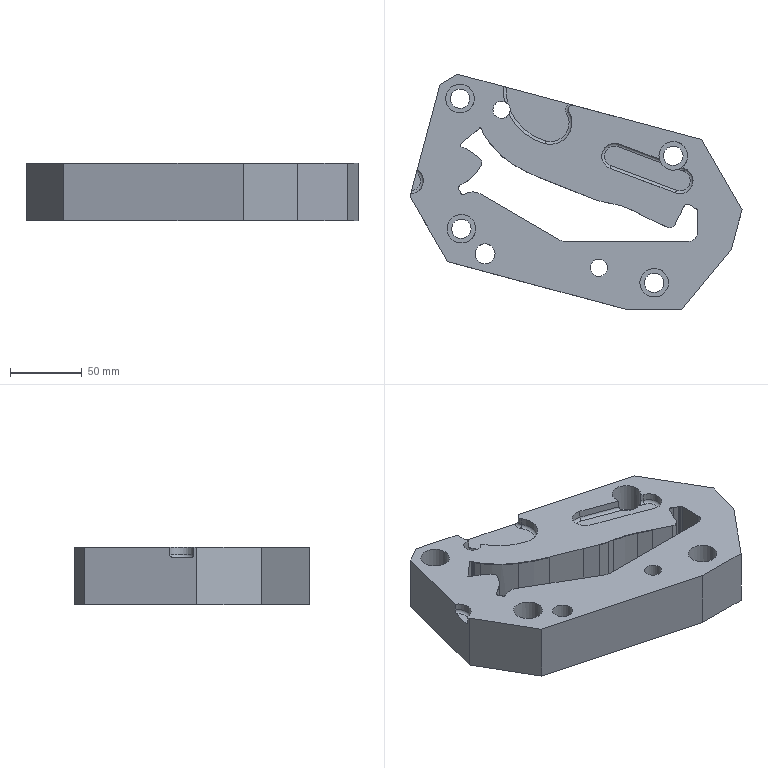Part | NX | features 23 2 | 1 solid | 124 faces | box 231.499 x 164.212 x 40 mm | volume 804818 mm3 | spline 44 | plane 40 | cylinder 33 | torus 7 | commonest cylinder face diameters 2 x8 20 x6 13.5 x4 4 x3 18.155 x3 12.001 x2